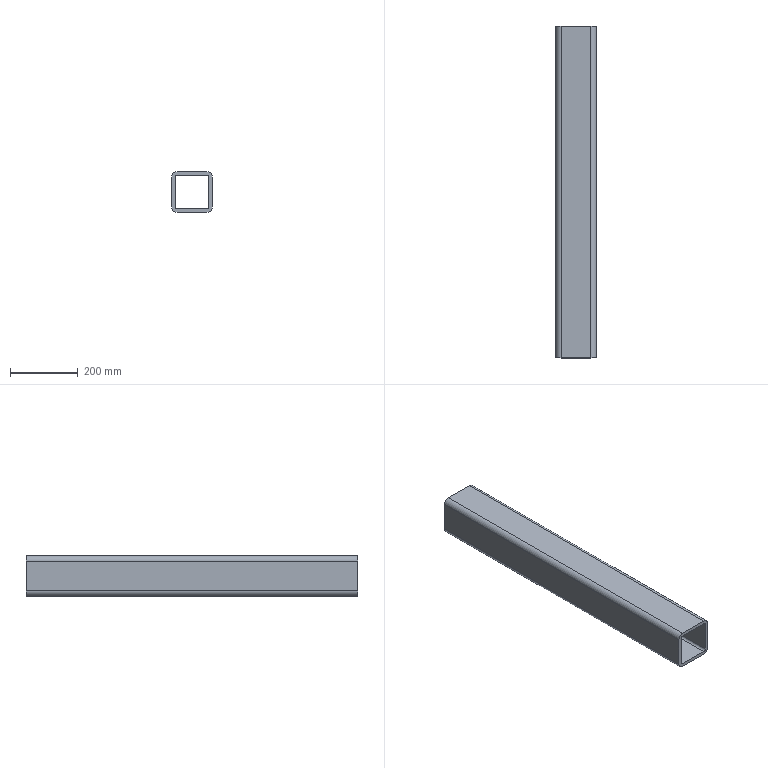Part | SolidWorks | features WeldMemberFeat 1, WeldmentFeature 1 | 1 solid | 18 faces | box 120 x 980 x 120 mm | volume 4126927 mm3 | plane 10 | cylinder 8 | commonest cylinder face diameters 12 x4 32 x4
STEP:
#1=CARTESIAN_POINT('',(-60.,0.,44.));
#2=VERTEX_POINT('',#1);
#3=CARTESIAN_POINT('',(-44.,0.,60.));
#4=VERTEX_POINT('',#3);
#5=CARTESIAN_POINT('',(-44.,0.,44.));
#6=DIRECTION('',(0.,1.,0.));
#7=DIRECTION('',(0.,0.,1.));
#8=AXIS2_PLACEMENT_3D('',#5,#6,#7);
#9=CIRCLE('',#8,16.);
#10=EDGE_CURVE('',#2,#4,#9,.T.);
#11=ORIENTED_EDGE('',*,*,#10,.T.);
#12=CARTESIAN_POINT('',(-44.,980.,60.));
#13=VERTEX_POINT('',#12);
#14=CARTESIAN_POINT('',(-44.,980.,60.));
#15=DIRECTION('',(0.,-1.,0.));
#16=VECTOR('',#15,1000.);
#17=LINE('',#14,#16);
#18=EDGE_CURVE('',#13,#4,#17,.T.);
#19=ORIENTED_EDGE('',*,*,#18,.F.);
#20=CARTESIAN_POINT('',(-60.,980.,44.));
#21=VERTEX_POINT('',#20);
#22=CARTESIAN_POINT('',(-44.,980.,44.));
#23=DIRECTION('',(0.,1.,0.));
#24=DIRECTION('',(0.,0.,1.));
#25=AXIS2_PLACEMENT_3D('',#22,#23,#24);
#26=CIRCLE('',#25,16.);
#27=EDGE_CURVE('',#21,#13,#26,.T.);
#28=ORIENTED_EDGE('',*,*,#27,.F.);
#29=CARTESIAN_POINT('',(-60.,980.,44.));
#30=DIRECTION('',(0.,-1.,0.));
#31=VECTOR('',#30,1000.);
#32=LINE('',#29,#31);
#33=EDGE_CURVE('',#21,#2,#32,.T.);
#34=ORIENTED_EDGE('',*,*,#33,.T.);
#35=EDGE_LOOP('',(#11,#19,#28,#34));
#36=FACE_OUTER_BOUND('',#35,.T.);
#37=CARTESIAN_POINT('',(-44.,980.,44.));
#38=DIRECTION('',(0.,-1.,0.));
#39=DIRECTION('',(0.,0.,-1.));
#40=AXIS2_PLACEMENT_3D('',#37,#38,#39);
#41=CYLINDRICAL_SURFACE('',#40,16.);
#42=ADVANCED_FACE('',(#36),#41,.T.);
#43=CARTESIAN_POINT('',(44.,0.,60.));
#44=VERTEX_POINT('',#43);
#45=CARTESIAN_POINT('',(-44.,0.,60.));
#46=DIRECTION('',(1.,0.,0.));
#47=VECTOR('',#46,1000.);
#48=LINE('',#45,#47);
#49=EDGE_CURVE('',#4,#44,#48,.T.);
#50=ORIENTED_EDGE('',*,*,#49,.T.);
#51=CARTESIAN_POINT('',(44.,980.,60.));
#52=VERTEX_POINT('',#51);
#53=CARTESIAN_POINT('',(44.,980.,60.));
#54=DIRECTION('',(0.,-1.,0.));
#55=VECTOR('',#54,1000.);
#56=LINE('',#53,#55);
#57=EDGE_CURVE('',#52,#44,#56,.T.);
#58=ORIENTED_EDGE('',*,*,#57,.F.);
#59=CARTESIAN_POINT('',(-44.,980.,60.));
#60=DIRECTION('',(1.,0.,0.));
#61=VECTOR('',#60,1000.);
#62=LINE('',#59,#61);
#63=EDGE_CURVE('',#13,#52,#62,.T.);
#64=ORIENTED_EDGE('',*,*,#63,.F.);
#65=ORIENTED_EDGE('',*,*,#18,.T.);
#66=EDGE_LOOP('',(#50,#58,#64,#65));
#67=FACE_OUTER_BOUND('',#66,.T.);
#68=CARTESIAN_POINT('',(-44.,980.,60.));
#69=DIRECTION('',(0.,0.,-1.));
#70=DIRECTION('',(-1.,0.,0.));
#71=AXIS2_PLACEMENT_3D('',#68,#69,#70);
#72=PLANE('',#71);
#73=ADVANCED_FACE('',(#67),#72,.F.);
#74=CARTESIAN_POINT('',(60.,0.,44.));
#75=VERTEX_POINT('',#74);
#76=CARTESIAN_POINT('',(44.,0.,44.));
#77=DIRECTION('',(0.,1.,0.));
#78=DIRECTION('',(0.,0.,1.));
#79=AXIS2_PLACEMENT_3D('',#76,#77,#78);
#80=CIRCLE('',#79,16.);
#81=EDGE_CURVE('',#44,#75,#80,.T.);
#82=ORIENTED_EDGE('',*,*,#81,.T.);
#83=CARTESIAN_POINT('',(60.,980.,44.));
#84=VERTEX_POINT('',#83);
#85=CARTESIAN_POINT('',(60.,980.,44.));
#86=DIRECTION('',(0.,-1.,0.));
#87=VECTOR('',#86,1000.);
#88=LINE('',#85,#87);
#89=EDGE_CURVE('',#84,#75,#88,.T.);
#90=ORIENTED_EDGE('',*,*,#89,.F.);
#91=CARTESIAN_POINT('',(44.,980.,44.));
#92=DIRECTION('',(0.,1.,0.));
#93=DIRECTION('',(0.,0.,1.));
#94=AXIS2_PLACEMENT_3D('',#91,#92,#93);
#95=CIRCLE('',#94,16.);
#96=EDGE_CURVE('',#52,#84,#95,.T.);
#97=ORIENTED_EDGE('',*,*,#96,.F.);
#98=ORIENTED_EDGE('',*,*,#57,.T.);
#99=EDGE_LOOP('',(#82,#90,#97,#98));
#100=FACE_OUTER_BOUND('',#99,.T.);
#101=CARTESIAN_POINT('',(44.,980.,44.));
#102=DIRECTION('',(0.,-1.,0.));
#103=DIRECTION('',(0.,0.,-1.));
#104=AXIS2_PLACEMENT_3D('',#101,#102,#103);
#105=CYLINDRICAL_SURFACE('',#104,16.);
#106=ADVANCED_FACE('',(#100),#105,.T.);
#107=CARTESIAN_POINT('',(60.,0.,-44.));
#108=VERTEX_POINT('',#107);
#109=CARTESIAN_POINT('',(60.,0.,-44.));
#110=DIRECTION('',(0.,0.,-1.));
#111=VECTOR('',#110,1000.);
#112=LINE('',#109,#111);
#113=EDGE_CURVE('',#75,#108,#112,.T.);
#114=ORIENTED_EDGE('',*,*,#113,.T.);
#115=CARTESIAN_POINT('',(60.,980.,-44.));
#116=VERTEX_POINT('',#115);
#117=CARTESIAN_POINT('',(60.,980.,-44.));
#118=DIRECTION('',(0.,-1.,0.));
#119=VECTOR('',#118,1000.);
#120=LINE('',#117,#119);
#121=EDGE_CURVE('',#116,#108,#120,.T.);
#122=ORIENTED_EDGE('',*,*,#121,.F.);
#123=CARTESIAN_POINT('',(60.,980.,-44.));
#124=DIRECTION('',(0.,0.,-1.));
#125=VECTOR('',#124,1000.);
#126=LINE('',#123,#125);
#127=EDGE_CURVE('',#84,#116,#126,.T.);
#128=ORIENTED_EDGE('',*,*,#127,.F.);
#129=ORIENTED_EDGE('',*,*,#89,.T.);
#130=EDGE_LOOP('',(#114,#122,#128,#129));
#131=FACE_OUTER_BOUND('',#130,.T.);
#132=CARTESIAN_POINT('',(60.,980.,-44.));
#133=DIRECTION('',(-1.,0.,0.));
#134=DIRECTION('',(0.,0.,1.));
#135=AXIS2_PLACEMENT_3D('',#132,#133,#134);
#136=PLANE('',#135);
#137=ADVANCED_FACE('',(#131),#136,.F.);
#138=CARTESIAN_POINT('',(44.,0.,-60.));
#139=VERTEX_POINT('',#138);
#140=CARTESIAN_POINT('',(44.,0.,-44.));
#141=DIRECTION('',(0.,1.,0.));
#142=DIRECTION('',(0.,0.,1.));
#143=AXIS2_PLACEMENT_3D('',#140,#141,#142);
#144=CIRCLE('',#143,16.);
#145=EDGE_CURVE('',#108,#139,#144,.T.);
#146=ORIENTED_EDGE('',*,*,#145,.T.);
#147=CARTESIAN_POINT('',(44.,980.,-60.));
#148=VERTEX_POINT('',#147);
#149=CARTESIAN_POINT('',(44.,980.,-60.));
#150=DIRECTION('',(0.,-1.,0.));
#151=VECTOR('',#150,1000.);
#152=LINE('',#149,#151);
#153=EDGE_CURVE('',#148,#139,#152,.T.);
#154=ORIENTED_EDGE('',*,*,#153,.F.);
#155=CARTESIAN_POINT('',(44.,980.,-44.));
#156=DIRECTION('',(0.,1.,0.));
#157=DIRECTION('',(0.,0.,1.));
#158=AXIS2_PLACEMENT_3D('',#155,#156,#157);
#159=CIRCLE('',#158,16.);
#160=EDGE_CURVE('',#116,#148,#159,.T.);
#161=ORIENTED_EDGE('',*,*,#160,.F.);
#162=ORIENTED_EDGE('',*,*,#121,.T.);
#163=EDGE_LOOP('',(#146,#154,#161,#162));
#164=FACE_OUTER_BOUND('',#163,.T.);
#165=CARTESIAN_POINT('',(44.,980.,-44.));
#166=DIRECTION('',(0.,-1.,0.));
#167=DIRECTION('',(0.,0.,-1.));
#168=AXIS2_PLACEMENT_3D('',#165,#166,#167);
#169=CYLINDRICAL_SURFACE('',#168,16.);
#170=ADVANCED_FACE('',(#164),#169,.T.);
#171=CARTESIAN_POINT('',(-44.,0.,-60.));
#172=VERTEX_POINT('',#171);
#173=CARTESIAN_POINT('',(44.,0.,-60.));
#174=DIRECTION('',(-1.,0.,0.));
#175=VECTOR('',#174,1000.);
#176=LINE('',#173,#175);
#177=EDGE_CURVE('',#139,#172,#176,.T.);
#178=ORIENTED_EDGE('',*,*,#177,.T.);
#179=CARTESIAN_POINT('',(-44.,980.,-60.));
#180=VERTEX_POINT('',#179);
#181=CARTESIAN_POINT('',(-44.,980.,-60.));
#182=DIRECTION('',(0.,-1.,0.));
#183=VECTOR('',#182,1000.);
#184=LINE('',#181,#183);
#185=EDGE_CURVE('',#180,#172,#184,.T.);
#186=ORIENTED_EDGE('',*,*,#185,.F.);
#187=CARTESIAN_POINT('',(44.,980.,-60.));
#188=DIRECTION('',(-1.,0.,0.));
#189=VECTOR('',#188,1000.);
#190=LINE('',#187,#189);
#191=EDGE_CURVE('',#148,#180,#190,.T.);
#192=ORIENTED_EDGE('',*,*,#191,.F.);
#193=ORIENTED_EDGE('',*,*,#153,.T.);
#194=EDGE_LOOP('',(#178,#186,#192,#193));
#195=FACE_OUTER_BOUND('',#194,.T.);
#196=CARTESIAN_POINT('',(44.,980.,-60.));
#197=DIRECTION('',(0.,0.,1.));
#198=DIRECTION('',(1.,0.,0.));
#199=AXIS2_PLACEMENT_3D('',#196,#197,#198);
#200=PLANE('',#199);
#201=ADVANCED_FACE('',(#195),#200,.F.);
#202=CARTESIAN_POINT('',(-60.,0.,-44.));
#203=VERTEX_POINT('',#202);
#204=CARTESIAN_POINT('',(-44.,0.,-44.));
#205=DIRECTION('',(0.,1.,0.));
#206=DIRECTION('',(0.,0.,1.));
#207=AXIS2_PLACEMENT_3D('',#204,#205,#206);
#208=CIRCLE('',#207,16.);
#209=EDGE_CURVE('',#172,#203,#208,.T.);
#210=ORIENTED_EDGE('',*,*,#209,.T.);
#211=CARTESIAN_POINT('',(-60.,980.,-44.));
#212=VERTEX_POINT('',#211);
#213=CARTESIAN_POINT('',(-60.,980.,-44.));
#214=DIRECTION('',(0.,-1.,0.));
#215=VECTOR('',#214,1000.);
#216=LINE('',#213,#215);
#217=EDGE_CURVE('',#212,#203,#216,.T.);
#218=ORIENTED_EDGE('',*,*,#217,.F.);
#219=CARTESIAN_POINT('',(-44.,980.,-44.));
#220=DIRECTION('',(0.,1.,0.));
#221=DIRECTION('',(0.,0.,1.));
#222=AXIS2_PLACEMENT_3D('',#219,#220,#221);
#223=CIRCLE('',#222,16.);
#224=EDGE_CURVE('',#180,#212,#223,.T.);
#225=ORIENTED_EDGE('',*,*,#224,.F.);
#226=ORIENTED_EDGE('',*,*,#185,.T.);
#227=EDGE_LOOP('',(#210,#218,#225,#226));
#228=FACE_OUTER_BOUND('',#227,.T.);
#229=CARTESIAN_POINT('',(-44.,980.,-44.));
#230=DIRECTION('',(0.,-1.,0.));
#231=DIRECTION('',(0.,0.,-1.));
#232=AXIS2_PLACEMENT_3D('',#229,#230,#231);
#233=CYLINDRICAL_SURFACE('',#232,16.);
#234=ADVANCED_FACE('',(#228),#233,.T.);
#235=CARTESIAN_POINT('',(44.,0.,50.));
#236=VERTEX_POINT('',#235);
#237=CARTESIAN_POINT('',(50.,0.,44.));
#238=VERTEX_POINT('',#237);
#239=CARTESIAN_POINT('',(44.,0.,44.));
#240=DIRECTION('',(0.,1.,0.));
#241=DIRECTION('',(0.,0.,1.));
#242=AXIS2_PLACEMENT_3D('',#239,#240,#241);
#243=CIRCLE('',#242,6.);
#244=EDGE_CURVE('',#236,#238,#243,.T.);
#245=ORIENTED_EDGE('',*,*,#244,.F.);
#246=CARTESIAN_POINT('',(44.,980.,50.));
#247=VERTEX_POINT('',#246);
#248=CARTESIAN_POINT('',(44.,980.,50.));
#249=DIRECTION('',(0.,-1.,0.));
#250=VECTOR('',#249,1000.);
#251=LINE('',#248,#250);
#252=EDGE_CURVE('',#247,#236,#251,.T.);
#253=ORIENTED_EDGE('',*,*,#252,.F.);
#254=CARTESIAN_POINT('',(50.,980.,44.));
#255=VERTEX_POINT('',#254);
#256=CARTESIAN_POINT('',(44.,980.,44.));
#257=DIRECTION('',(0.,1.,0.));
#258=DIRECTION('',(0.,0.,1.));
#259=AXIS2_PLACEMENT_3D('',#256,#257,#258);
#260=CIRCLE('',#259,6.);
#261=EDGE_CURVE('',#247,#255,#260,.T.);
#262=ORIENTED_EDGE('',*,*,#261,.T.);
#263=CARTESIAN_POINT('',(50.,980.,44.));
#264=DIRECTION('',(0.,-1.,0.));
#265=VECTOR('',#264,1000.);
#266=LINE('',#263,#265);
#267=EDGE_CURVE('',#255,#238,#266,.T.);
#268=ORIENTED_EDGE('',*,*,#267,.T.);
#269=EDGE_LOOP('',(#245,#253,#262,#268));
#270=FACE_OUTER_BOUND('',#269,.T.);
#271=CARTESIAN_POINT('',(44.,980.,44.));
#272=DIRECTION('',(0.,-1.,0.));
#273=DIRECTION('',(0.,0.,-1.));
#274=AXIS2_PLACEMENT_3D('',#271,#272,#273);
#275=CYLINDRICAL_SURFACE('',#274,6.);
#276=ADVANCED_FACE('',(#270),#275,.F.);
#277=CARTESIAN_POINT('',(-44.,0.,50.));
#278=VERTEX_POINT('',#277);
#279=CARTESIAN_POINT('',(-44.,0.,50.));
#280=DIRECTION('',(1.,0.,0.));
#281=VECTOR('',#280,1000.);
#282=LINE('',#279,#281);
#283=EDGE_CURVE('',#278,#236,#282,.T.);
#284=ORIENTED_EDGE('',*,*,#283,.F.);
#285=CARTESIAN_POINT('',(-44.,980.,50.));
#286=VERTEX_POINT('',#285);
#287=CARTESIAN_POINT('',(-44.,980.,50.));
#288=DIRECTION('',(0.,-1.,0.));
#289=VECTOR('',#288,1000.);
#290=LINE('',#287,#289);
#291=EDGE_CURVE('',#286,#278,#290,.T.);
#292=ORIENTED_EDGE('',*,*,#291,.F.);
#293=CARTESIAN_POINT('',(-44.,980.,50.));
#294=DIRECTION('',(1.,0.,0.));
#295=VECTOR('',#294,1000.);
#296=LINE('',#293,#295);
#297=EDGE_CURVE('',#286,#247,#296,.T.);
#298=ORIENTED_EDGE('',*,*,#297,.T.);
#299=ORIENTED_EDGE('',*,*,#252,.T.);
#300=EDGE_LOOP('',(#284,#292,#298,#299));
#301=FACE_OUTER_BOUND('',#300,.T.);
#302=CARTESIAN_POINT('',(-44.,980.,50.));
#303=DIRECTION('',(0.,0.,-1.));
#304=DIRECTION('',(-1.,0.,0.));
#305=AXIS2_PLACEMENT_3D('',#302,#303,#304);
#306=PLANE('',#305);
#307=ADVANCED_FACE('',(#301),#306,.T.);
#308=CARTESIAN_POINT('',(-50.,0.,44.));
#309=VERTEX_POINT('',#308);
#310=CARTESIAN_POINT('',(-44.,0.,44.));
#311=DIRECTION('',(0.,1.,0.));
#312=DIRECTION('',(0.,0.,1.));
#313=AXIS2_PLACEMENT_3D('',#310,#311,#312);
#314=CIRCLE('',#313,6.);
#315=EDGE_CURVE('',#309,#278,#314,.T.);
#316=ORIENTED_EDGE('',*,*,#315,.F.);
#317=CARTESIAN_POINT('',(-50.,980.,44.));
#318=VERTEX_POINT('',#317);
#319=CARTESIAN_POINT('',(-50.,980.,44.));
#320=DIRECTION('',(0.,-1.,0.));
#321=VECTOR('',#320,1000.);
#322=LINE('',#319,#321);
#323=EDGE_CURVE('',#318,#309,#322,.T.);
#324=ORIENTED_EDGE('',*,*,#323,.F.);
#325=CARTESIAN_POINT('',(-44.,980.,44.));
#326=DIRECTION('',(0.,1.,0.));
#327=DIRECTION('',(0.,0.,1.));
#328=AXIS2_PLACEMENT_3D('',#325,#326,#327);
#329=CIRCLE('',#328,6.);
#330=EDGE_CURVE('',#318,#286,#329,.T.);
#331=ORIENTED_EDGE('',*,*,#330,.T.);
#332=ORIENTED_EDGE('',*,*,#291,.T.);
#333=EDGE_LOOP('',(#316,#324,#331,#332));
#334=FACE_OUTER_BOUND('',#333,.T.);
#335=CARTESIAN_POINT('',(-44.,980.,44.));
#336=DIRECTION('',(0.,-1.,0.));
#337=DIRECTION('',(0.,0.,-1.));
#338=AXIS2_PLACEMENT_3D('',#335,#336,#337);
#339=CYLINDRICAL_SURFACE('',#338,6.);
#340=ADVANCED_FACE('',(#334),#339,.F.);
#341=CARTESIAN_POINT('',(-50.,0.,-44.));
#342=VERTEX_POINT('',#341);
#343=CARTESIAN_POINT('',(-50.,0.,44.));
#344=DIRECTION('',(0.,0.,1.));
#345=VECTOR('',#344,1000.);
#346=LINE('',#343,#345);
#347=EDGE_CURVE('',#342,#309,#346,.T.);
#348=ORIENTED_EDGE('',*,*,#347,.F.);
#349=CARTESIAN_POINT('',(-50.,980.,-44.));
#350=VERTEX_POINT('',#349);
#351=CARTESIAN_POINT('',(-50.,980.,-44.));
#352=DIRECTION('',(0.,-1.,0.));
#353=VECTOR('',#352,1000.);
#354=LINE('',#351,#353);
#355=EDGE_CURVE('',#350,#342,#354,.T.);
#356=ORIENTED_EDGE('',*,*,#355,.F.);
#357=CARTESIAN_POINT('',(-50.,980.,44.));
#358=DIRECTION('',(0.,0.,1.));
#359=VECTOR('',#358,1000.);
#360=LINE('',#357,#359);
#361=EDGE_CURVE('',#350,#318,#360,.T.);
#362=ORIENTED_EDGE('',*,*,#361,.T.);
#363=ORIENTED_EDGE('',*,*,#323,.T.);
#364=EDGE_LOOP('',(#348,#356,#362,#363));
#365=FACE_OUTER_BOUND('',#364,.T.);
#366=CARTESIAN_POINT('',(-50.,980.,44.));
#367=DIRECTION('',(1.,0.,0.));
#368=DIRECTION('',(0.,0.,-1.));
#369=AXIS2_PLACEMENT_3D('',#366,#367,#368);
#370=PLANE('',#369);
#371=ADVANCED_FACE('',(#365),#370,.T.);
#372=CARTESIAN_POINT('',(-44.,0.,-50.));
#373=VERTEX_POINT('',#372);
#374=CARTESIAN_POINT('',(-44.,0.,-44.));
#375=DIRECTION('',(0.,1.,0.));
#376=DIRECTION('',(0.,0.,1.));
#377=AXIS2_PLACEMENT_3D('',#374,#375,#376);
#378=CIRCLE('',#377,6.);
#379=EDGE_CURVE('',#373,#342,#378,.T.);
#380=ORIENTED_EDGE('',*,*,#379,.F.);
#381=CARTESIAN_POINT('',(-44.,980.,-50.));
#382=VERTEX_POINT('',#381);
#383=CARTESIAN_POINT('',(-44.,980.,-50.));
#384=DIRECTION('',(0.,-1.,0.));
#385=VECTOR('',#384,1000.);
#386=LINE('',#383,#385);
#387=EDGE_CURVE('',#382,#373,#386,.T.);
#388=ORIENTED_EDGE('',*,*,#387,.F.);
#389=CARTESIAN_POINT('',(-44.,980.,-44.));
#390=DIRECTION('',(0.,1.,0.));
#391=DIRECTION('',(0.,0.,1.));
#392=AXIS2_PLACEMENT_3D('',#389,#390,#391);
#393=CIRCLE('',#392,6.);
#394=EDGE_CURVE('',#382,#350,#393,.T.);
#395=ORIENTED_EDGE('',*,*,#394,.T.);
#396=ORIENTED_EDGE('',*,*,#355,.T.);
#397=EDGE_LOOP('',(#380,#388,#395,#396));
#398=FACE_OUTER_BOUND('',#397,.T.);
#399=CARTESIAN_POINT('',(-44.,980.,-44.));
#400=DIRECTION('',(0.,-1.,0.));
#401=DIRECTION('',(0.,0.,-1.));
#402=AXIS2_PLACEMENT_3D('',#399,#400,#401);
#403=CYLINDRICAL_SURFACE('',#402,6.);
#404=ADVANCED_FACE('',(#398),#403,.F.);
#405=CARTESIAN_POINT('',(44.,0.,-50.));
#406=VERTEX_POINT('',#405);
#407=CARTESIAN_POINT('',(44.,0.,-50.));
#408=DIRECTION('',(-1.,0.,0.));
#409=VECTOR('',#408,1000.);
#410=LINE('',#407,#409);
#411=EDGE_CURVE('',#406,#373,#410,.T.);
#412=ORIENTED_EDGE('',*,*,#411,.F.);
#413=CARTESIAN_POINT('',(44.,980.,-50.));
#414=VERTEX_POINT('',#413);
#415=CARTESIAN_POINT('',(44.,980.,-50.));
#416=DIRECTION('',(0.,-1.,0.));
#417=VECTOR('',#416,1000.);
#418=LINE('',#415,#417);
#419=EDGE_CURVE('',#414,#406,#418,.T.);
#420=ORIENTED_EDGE('',*,*,#419,.F.);
#421=CARTESIAN_POINT('',(44.,980.,-50.));
#422=DIRECTION('',(-1.,0.,0.));
#423=VECTOR('',#422,1000.);
#424=LINE('',#421,#423);
#425=EDGE_CURVE('',#414,#382,#424,.T.);
#426=ORIENTED_EDGE('',*,*,#425,.T.);
#427=ORIENTED_EDGE('',*,*,#387,.T.);
#428=EDGE_LOOP('',(#412,#420,#426,#427));
#429=FACE_OUTER_BOUND('',#428,.T.);
#430=CARTESIAN_POINT('',(44.,980.,-50.));
#431=DIRECTION('',(0.,0.,1.));
#432=DIRECTION('',(1.,0.,0.));
#433=AXIS2_PLACEMENT_3D('',#430,#431,#432);
#434=PLANE('',#433);
#435=ADVANCED_FACE('',(#429),#434,.T.);
#436=CARTESIAN_POINT('',(50.,0.,-44.));
#437=VERTEX_POINT('',#436);
#438=CARTESIAN_POINT('',(44.,0.,-44.));
#439=DIRECTION('',(0.,1.,0.));
#440=DIRECTION('',(0.,0.,1.));
#441=AXIS2_PLACEMENT_3D('',#438,#439,#440);
#442=CIRCLE('',#441,6.);
#443=EDGE_CURVE('',#437,#406,#442,.T.);
#444=ORIENTED_EDGE('',*,*,#443,.F.);
#445=CARTESIAN_POINT('',(50.,980.,-44.));
#446=VERTEX_POINT('',#445);
#447=CARTESIAN_POINT('',(50.,980.,-44.));
#448=DIRECTION('',(0.,-1.,0.));
#449=VECTOR('',#448,1000.);
#450=LINE('',#447,#449);
#451=EDGE_CURVE('',#446,#437,#450,.T.);
#452=ORIENTED_EDGE('',*,*,#451,.F.);
#453=CARTESIAN_POINT('',(44.,980.,-44.));
#454=DIRECTION('',(0.,1.,0.));
#455=DIRECTION('',(0.,0.,1.));
#456=AXIS2_PLACEMENT_3D('',#453,#454,#455);
#457=CIRCLE('',#456,6.);
#458=EDGE_CURVE('',#446,#414,#457,.T.);
#459=ORIENTED_EDGE('',*,*,#458,.T.);
#460=ORIENTED_EDGE('',*,*,#419,.T.);
#461=EDGE_LOOP('',(#444,#452,#459,#460));
#462=FACE_OUTER_BOUND('',#461,.T.);
#463=CARTESIAN_POINT('',(44.,980.,-44.));
#464=DIRECTION('',(0.,-1.,0.));
#465=DIRECTION('',(0.,0.,-1.));
#466=AXIS2_PLACEMENT_3D('',#463,#464,#465);
#467=CYLINDRICAL_SURFACE('',#466,6.);
#468=ADVANCED_FACE('',(#462),#467,.F.);
#469=CARTESIAN_POINT('',(50.,0.,-44.));
#470=DIRECTION('',(0.,0.,-1.));
#471=VECTOR('',#470,1000.);
#472=LINE('',#469,#471);
#473=EDGE_CURVE('',#238,#437,#472,.T.);
#474=ORIENTED_EDGE('',*,*,#473,.F.);
#475=ORIENTED_EDGE('',*,*,#267,.F.);
#476=CARTESIAN_POINT('',(50.,980.,-44.));
#477=DIRECTION('',(0.,0.,-1.));
#478=VECTOR('',#477,1000.);
#479=LINE('',#476,#478);
#480=EDGE_CURVE('',#255,#446,#479,.T.);
#481=ORIENTED_EDGE('',*,*,#480,.T.);
#482=ORIENTED_EDGE('',*,*,#451,.T.);
#483=EDGE_LOOP('',(#474,#475,#481,#482));
#484=FACE_OUTER_BOUND('',#483,.T.);
#485=CARTESIAN_POINT('',(50.,980.,-44.));
#486=DIRECTION('',(-1.,0.,0.));
#487=DIRECTION('',(0.,0.,1.));
#488=AXIS2_PLACEMENT_3D('',#485,#486,#487);
#489=PLANE('',#488);
#490=ADVANCED_FACE('',(#484),#489,.T.);
#491=CARTESIAN_POINT('',(-60.,0.,44.));
#492=DIRECTION('',(0.,0.,1.));
#493=VECTOR('',#492,1000.);
#494=LINE('',#491,#493);
#495=EDGE_CURVE('',#203,#2,#494,.T.);
#496=ORIENTED_EDGE('',*,*,#495,.T.);
#497=ORIENTED_EDGE('',*,*,#33,.F.);
#498=CARTESIAN_POINT('',(-60.,980.,44.));
#499=DIRECTION('',(0.,0.,1.));
#500=VECTOR('',#499,1000.);
#501=LINE('',#498,#500);
#502=EDGE_CURVE('',#212,#21,#501,.T.);
#503=ORIENTED_EDGE('',*,*,#502,.F.);
#504=ORIENTED_EDGE('',*,*,#217,.T.);
#505=EDGE_LOOP('',(#496,#497,#503,#504));
#506=FACE_OUTER_BOUND('',#505,.T.);
#507=CARTESIAN_POINT('',(-60.,980.,44.));
#508=DIRECTION('',(1.,0.,0.));
#509=DIRECTION('',(0.,0.,-1.));
#510=AXIS2_PLACEMENT_3D('',#507,#508,#509);
#511=PLANE('',#510);
#512=ADVANCED_FACE('',(#506),#511,.F.);
#513=ORIENTED_EDGE('',*,*,#261,.F.);
#514=ORIENTED_EDGE('',*,*,#297,.F.);
#515=ORIENTED_EDGE('',*,*,#330,.F.);
#516=ORIENTED_EDGE('',*,*,#361,.F.);
#517=ORIENTED_EDGE('',*,*,#394,.F.);
#518=ORIENTED_EDGE('',*,*,#425,.F.);
#519=ORIENTED_EDGE('',*,*,#458,.F.);
#520=ORIENTED_EDGE('',*,*,#480,.F.);
#521=EDGE_LOOP('',(#513,#514,#515,#516,#517,#518,#519,#520));
#522=FACE_BOUND('',#521,.T.);
#523=ORIENTED_EDGE('',*,*,#27,.T.);
#524=ORIENTED_EDGE('',*,*,#63,.T.);
#525=ORIENTED_EDGE('',*,*,#96,.T.);
#526=ORIENTED_EDGE('',*,*,#127,.T.);
#527=ORIENTED_EDGE('',*,*,#160,.T.);
#528=ORIENTED_EDGE('',*,*,#191,.T.);
#529=ORIENTED_EDGE('',*,*,#224,.T.);
#530=ORIENTED_EDGE('',*,*,#502,.T.);
#531=EDGE_LOOP('',(#523,#524,#525,#526,#527,#528,#529,#530));
#532=FACE_OUTER_BOUND('',#531,.T.);
#533=CARTESIAN_POINT('',(-44.,980.,44.));
#534=DIRECTION('',(0.,1.,0.));
#535=DIRECTION('',(0.,0.,1.));
#536=AXIS2_PLACEMENT_3D('',#533,#534,#535);
#537=PLANE('',#536);
#538=ADVANCED_FACE('',(#522,#532),#537,.T.);
#539=ORIENTED_EDGE('',*,*,#244,.T.);
#540=ORIENTED_EDGE('',*,*,#473,.T.);
#541=ORIENTED_EDGE('',*,*,#443,.T.);
#542=ORIENTED_EDGE('',*,*,#411,.T.);
#543=ORIENTED_EDGE('',*,*,#379,.T.);
#544=ORIENTED_EDGE('',*,*,#347,.T.);
#545=ORIENTED_EDGE('',*,*,#315,.T.);
#546=ORIENTED_EDGE('',*,*,#283,.T.);
#547=EDGE_LOOP('',(#539,#540,#541,#542,#543,#544,#545,#546));
#548=FACE_BOUND('',#547,.T.);
#549=ORIENTED_EDGE('',*,*,#10,.F.);
#550=ORIENTED_EDGE('',*,*,#495,.F.);
#551=ORIENTED_EDGE('',*,*,#209,.F.);
#552=ORIENTED_EDGE('',*,*,#177,.F.);
#553=ORIENTED_EDGE('',*,*,#145,.F.);
#554=ORIENTED_EDGE('',*,*,#113,.F.);
#555=ORIENTED_EDGE('',*,*,#81,.F.);
#556=ORIENTED_EDGE('',*,*,#49,.F.);
#557=EDGE_LOOP('',(#549,#550,#551,#552,#553,#554,#555,#556));
#558=FACE_OUTER_BOUND('',#557,.T.);
#559=CARTESIAN_POINT('',(-44.,0.,44.));
#560=DIRECTION('',(0.,1.,0.));
#561=DIRECTION('',(0.,0.,1.));
#562=AXIS2_PLACEMENT_3D('',#559,#560,#561);
#563=PLANE('',#562);
#564=ADVANCED_FACE('',(#548,#558),#563,.F.);
#565=CLOSED_SHELL('',(#42,#73,#106,#137,#170,#201,#234,#276,#307,#340,#371,#404,#435,#468,#490,#512,#538,#564));
#566=MANIFOLD_SOLID_BREP('',#565);
#567=CARTESIAN_POINT('',(0.,0.,0.));
#568=DIRECTION('',(0.,0.,1.));
#569=DIRECTION('',(1.,0.,0.));
#570=AXIS2_PLACEMENT_3D('',#567,#568,#569);
#571=(LENGTH_UNIT()NAMED_UNIT(*)SI_UNIT(.MILLI.,.METRE.));
#572=UNCERTAINTY_MEASURE_WITH_UNIT(LENGTH_MEASURE(0.00001),#571,'','');
#573=(NAMED_UNIT(*)PLANE_ANGLE_UNIT()SI_UNIT($,.RADIAN.));
#574=(NAMED_UNIT(*)SI_UNIT($,.STERADIAN.)SOLID_ANGLE_UNIT());
#575=(GEOMETRIC_REPRESENTATION_CONTEXT(3)GLOBAL_UNCERTAINTY_ASSIGNED_CONTEXT((#572))GLOBAL_UNIT_ASSIGNED_CONTEXT((#571,#573,#574))REPRESENTATION_CONTEXT('',''));
#576=ADVANCED_BREP_SHAPE_REPRESENTATION('',(#566,#570),#575);